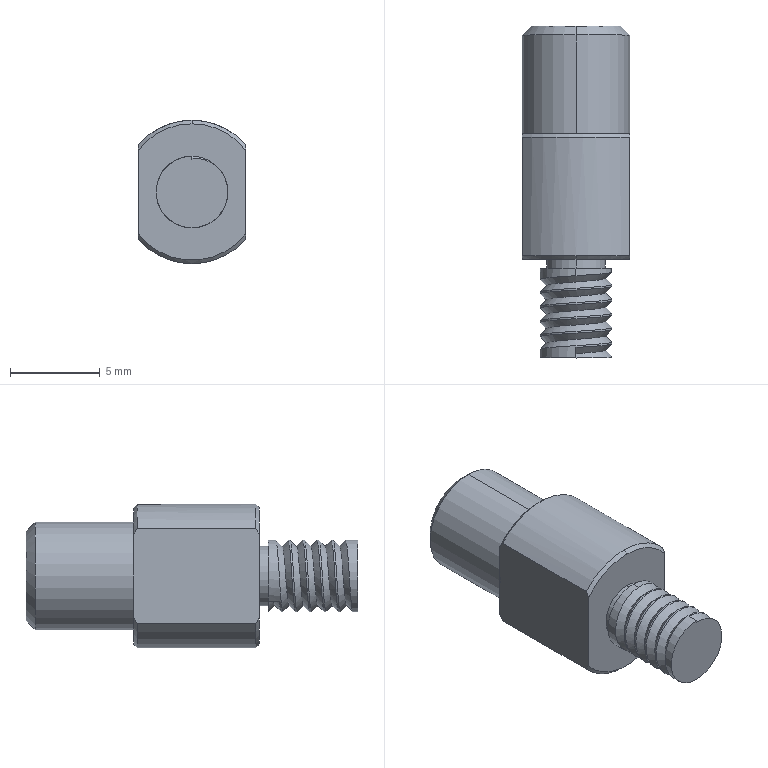Part | SolidWorks | features ICE 4, Chamfer 2, Extrusion 1, Helix 1, HoleWzd 1, SweepCut 1 | 1 solid | 45 faces | box 6 x 18.5 x 8 mm | volume 437.837 mm3 | cylinder 23 | cone 10 | plane 10 | spline 2 | commonest cylinder face diameters 4 x14 3.3 x4 8 x3 6 x2